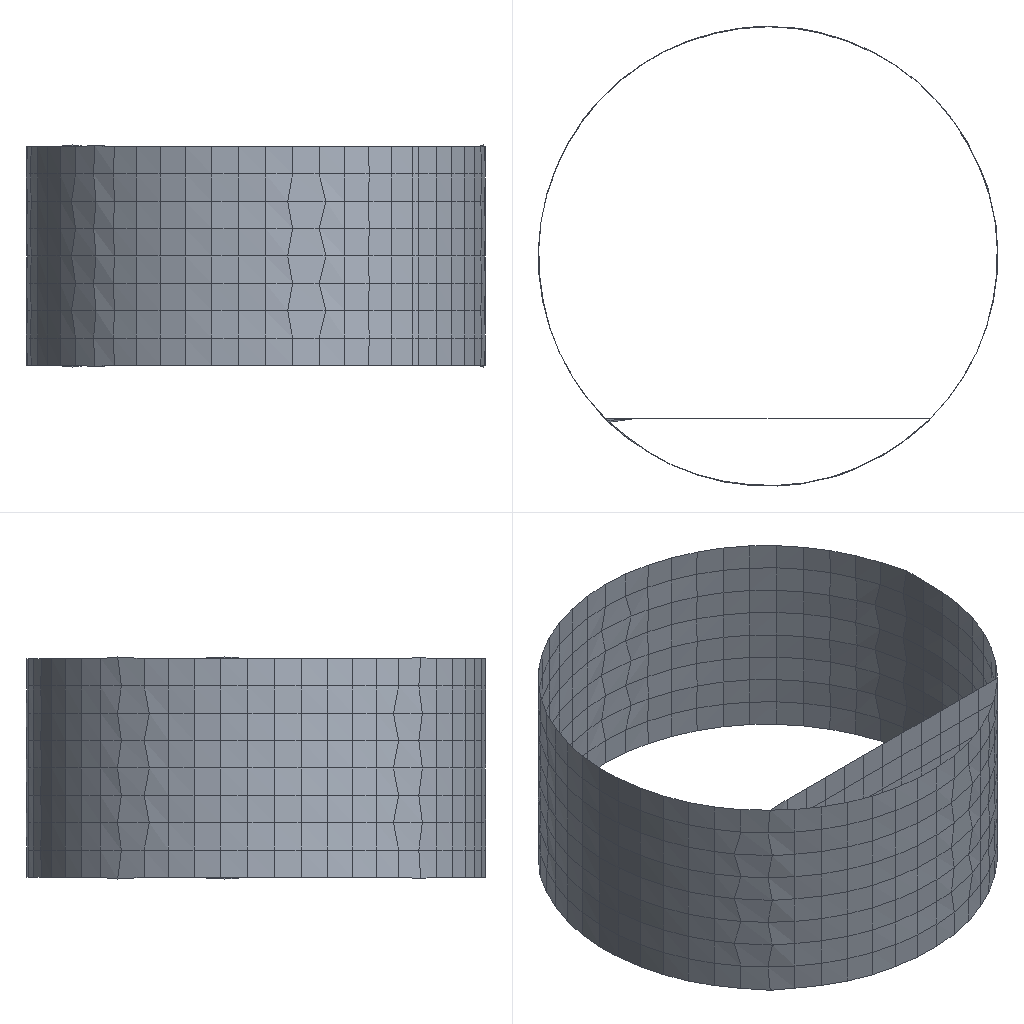Simulation study | abaqus
Set-up summary:
category,name,step,type,value,unit,region
solver,abaqus
solver,version,,,Abaqus/Standard 2020
units,not stated in the deck,,not stated
analysis,deck,,static,static
load_step,Step-1,Step-1,static
load_step,requested,,,1
mesh,nodes,,,1052
mesh,elements,,,966
element_type,B31,,beam,438
element_type,S4R,,shell,528
load,load commands in deck,,count,2
bc,support commands in deck,,count,1
material,FLOOR,,in results
material,FLOOR-STIFFENERS,,in results
material,FRAME,,in results
material,SKIN,,in results
material,STRINGER,,in results
check,setup vs results,,match,"per instance, exact: element labels, types and connectivity; labels of the nodes the elements use; coordinates of those nodes at SINGLE_PRECISION in 17 of 35 instance(s)"
Abaqus input file, long lists of numbers shortened:
*Heading
** Job name: Job-1 Model name: Model-1
** Generated by: Abaqus/CAE 2020
*Preprint, echo=NO, model=NO, history=NO, contact=NO
**
** PARTS
**
*Part, name=Part-1
*Node
      1,  -1484.924,  -1484.924,        2000.
      2,  -1484.924,  -1484.924,           0.
** (583 more lines like these left out)
*Element, type=S4R
  1,   1,   7, 145,  44
  2,   7,   8, 146, 145
** (526 more lines like these left out)
*Nset, nset=Set-1
   1,   2,   3,   4,   5,   6,   7,   8,   9,  10,  11,  12,  13,  14,  15,  16
  17,  18,  19,  20,  21,  22,  23,  24,  25,  26,  27,  28,  29,  30,  31,  32
** (29 more lines like these left out)
*Elset, elset=Set-1, generate
   1,  432,    1
*Nset, nset=Set-2
   1,   2,   4,   6,   7,   8,   9,  10,  11,  12,  13,  26,  27,  28,  29,  30
  31,  32, 123, 124, 125, 126, 127, 128, 129, 130, 131, 132, 133, 134, 135, 136
** (6 more lines like these left out)
*Elset, elset=Set-2, generate
 433,  528,    1
** Section: skin
*Shell Section, elset=Set-1, material=skin
2., 5
** Section: skin
*Shell Section, elset=Set-2, material=skin
2., 5
*End Part
**
*Part, name=floor-stiff
*Node
      1,       -1970.,           0.,           0.
      2,       -1673.,           0.,           0.
** (9 more lines like these left out)
*Element, type=B31
 1,  1,  2
 2,  2,  3
** (8 more lines like these left out)
*Nset, nset=Set-1, generate
  1,  11,   1
*Elset, elset=Set-1, generate
  1,  10,   1
*Nset, nset=Set-3, generate
  1,  11,   1
*Elset, elset=Set-3, generate
  1,  10,   1
** Section: floor-stiff  Profile: Profile-1
*Beam Section, elset=Set-1, material=floor-stiffeners, temperature=GRADIENTS, section=I
0., 50., 40., 30., 4., 4., 4.
0.,0.,-1.
*End Part
**
*Part, name=ring-frame5
*Node
      1,   1763.097,  -1140.828,           0.
      2,    1907.508,  -878.301,           0.
** (42 more lines like these left out)
*Element, type=B31
 1,  1,  2
 2,  2,  3
** (42 more lines like these left out)
*Nset, nset=Set-1, generate
  1,  44,   1
*Elset, elset=Set-1, generate
  1,  44,   1
*Nset, nset=Set-3, generate
  1,  44,   1
*Elset, elset=Set-3, generate
  1,  44,   1
** Section: frame  Profile: frame
*Beam Section, elset=Set-1, material=frame, temperature=GRADIENTS, section=ARBITRARY
3, 50., 158.5, 48.5, 158.5, 3.
1.5, 1.5, 3.
50., 1.5, 3.
0.,0.,-1.
*End Part
**
*Part, name=stringer
*Node
      1,        -600.,           0.,           0.
      2,  -314.286,           0.,           0.
** (6 more lines like these left out)
*Element, type=B31
1, 1, 2
2, 2, 3
** (5 more lines like these left out)
*Nset, nset=Set-1, generate
 1,  8,  1
*Elset, elset=Set-1, generate
 1,  7,  1
*Nset, nset=Set-2, generate
 1,  8,  1
*Elset, elset=Set-2, generate
 1,  7,  1
*Nset, nset=Set-3, generate
 1,  8,  1
*Elset, elset=Set-3, generate
 1,  7,  1
** Section: stringer  Profile: stringer
*Beam Section, elset=Set-1, material=stringer, temperature=GRADIENTS, section=ARBITRARY
3, -22., 35.5, 1., 35.5, 3.
1., -1.5, 2.
24., -1.5, 3.
0.,0.,-1.
*End Part
**
**
** ASSEMBLY
**
*Assembly, name=Assembly
**
*Instance, name=ring-frame5-1, part=ring-frame5
*End Instance
**
*Instance, name=Part-1-1, part=Part-1
*End Instance
**
*Instance, name=ring-frame5-1-lin-2-1, part=ring-frame5
          0.,           0.,         500.
*End Instance
**
*Instance, name=ring-frame5-1-lin-3-1, part=ring-frame5
          0.,           0.,        1000.
*End Instance
**
*Instance, name=ring-frame5-1-lin-4-1, part=ring-frame5
          0.,           0.,        1500.
*End Instance
**
*Instance, name=ring-frame5-1-lin-5-1, part=ring-frame5
          0.,           0.,        2000.
*End Instance
**
*Instance, name=stringer-1, part=stringer
 -1763.097,  1140.828,        1400.
 -1763.097,  1140.828,        1400.,  -1763.097, 1141.828,        1400., 90.
*End Instance
**
*Instance, name=stringer-1-rad-2, part=stringer
-1998.289, 645.632,        1400.
-1998.289, 645.632,        1400., -1998.419, 646.615, 1400.129, 90.976
*End Instance
**
*Instance, name=stringer-1-rad-3, part=stringer
-2097.301, 106.437,        1400.
-2097.301, 106.437,        1400., -2097.551, 107.372, 1400.251, 93.841
*End Instance
**
*Instance, name=stringer-1-rad-4, part=stringer
-2053.385, -440.011,        1400.
-2053.385, -440.011,        1400., -2053.742, -439.148, 1400.357, 98.421
*End Instance
**
*Instance, name=stringer-1-rad-5, part=stringer
-1869.534, -956.473,        1400.
-1869.534, -956.473,        1400., -1869.982, -955.699, 1400.447, 104.478
*End Instance
**
*Instance, name=stringer-1-rad-6, part=stringer
-1558.278, -1407.753,        1400.
-1558.278, -1407.753,        1400., -1558.798, -1407.076, 1400.52, 111.752
*End Instance
**
*Instance, name=stringer-1-rad-7, part=stringer
-1140.828,  -1763.097,        1400.
-1140.828,  -1763.097,        1400., -1141.405, -1762.52, 1400.577,         120.
*End Instance
**
*Instance, name=stringer-1-rad-8, part=stringer
-645.632, -1998.289,        1400.
-645.632, -1998.289,        1400., -646.253, -1997.812, 1400.622, 129.007
*End Instance
**
*Instance, name=stringer-1-rad-9, part=stringer
-106.437, -2097.301,        1400.
-106.437, -2097.301,        1400., -107.092, -2096.923, 1400.655, 138.59
*End Instance
**
*Instance, name=stringer-1-rad-10, part=stringer
440.011, -2053.385,        1400.
440.011, -2053.385,        1400., 439.332, -2053.104, 1400.679, 148.6
*End Instance
**
*Instance, name=stringer-1-rad-11, part=stringer
956.473, -1869.534,        1400.
956.473, -1869.534,        1400., 955.778, -1869.348, 1400.695, 158.909
*End Instance
**
*Instance, name=stringer-1-rad-12, part=stringer
1407.753, -1558.278,        1400.
1407.753, -1558.278,        1400., 1407.049, -1558.185, 1400.704, 169.409
*End Instance
**
*Instance, name=stringer-1-rad-13, part=stringer
  1763.097, -1140.828,        1400.
  1763.097, -1140.828,        1400., 1762.39, -1140.828, 1400.707,         180.
*End Instance
**
*Instance, name=stringer-1-rad-14, part=stringer
1998.289, -645.632,        1400.
1998.289, -645.632,        1400., 1997.585, -645.724, 1400.704, 190.591
*End Instance
**
*Instance, name=stringer-1-rad-15, part=stringer
2097.301, -106.437,        1400.
2097.301, -106.437,        1400., 2096.606, -106.623, 1400.695, 201.091
*End Instance
**
*Instance, name=stringer-1-rad-16, part=stringer
2053.385, 440.011,        1400.
2053.385, 440.011,        1400., 2052.706, 439.73, 1400.679, 211.4
*End Instance
**
*Instance, name=stringer-1-rad-17, part=stringer
1869.534, 956.473,        1400.
1869.534, 956.473,        1400., 1868.88, 956.095, 1400.655, 221.41
*End Instance
**
*Instance, name=stringer-1-rad-18, part=stringer
1558.278, 1407.753,        1400.
1558.278, 1407.753,        1400., 1557.657, 1407.276, 1400.622, 230.993
*End Instance
**
*Instance, name=stringer-1-rad-19, part=stringer
 1140.828,   1763.097,        1400.
 1140.828,   1763.097,        1400., 1140.25, 1762.52, 1400.577,         240.
*End Instance
**
*Instance, name=stringer-1-rad-20, part=stringer
645.632, 1998.289,        1400.
645.632, 1998.289,        1400., 646.152, 1998.967, 1399.48, 111.752
*End Instance
**
*Instance, name=stringer-1-rad-21, part=stringer
106.437, 2097.301,        1400.
106.437, 2097.301,        1400., 106.884, 2098.076, 1399.553, 104.478
*End Instance
**
*Instance, name=stringer-1-rad-22, part=stringer
-440.011, 2053.385,        1400.
-440.011, 2053.385,        1400., -439.654, 2054.248, 1399.643, 98.421
*End Instance
**
*Instance, name=stringer-1-rad-23, part=stringer
-956.473, 1869.534,        1400.
-956.473, 1869.534,        1400., -956.223, 1870.47, 1399.749, 93.841
*End Instance
**
*Instance, name=stringer-1-rad-24, part=stringer
-1407.753, 1558.278,        1400.
-1407.753, 1558.278,        1400., -1407.624, 1559.261, 1399.871, 90.976
*End Instance
**
*Instance, name=floor-stiff-1, part=floor-stiff
   485.076,  -1484.924,        2000.
*End Instance
**
*Instance, name=floor-stiff-1-lin-2-1, part=floor-stiff
   485.076,  -1484.924,        1500.
*End Instance
**
*Instance, name=floor-stiff-1-lin-3-1, part=floor-stiff
   485.076,  -1484.924,        1000.
*End Instance
**
*Instance, name=floor-stiff-1-lin-4-1, part=floor-stiff
   485.076,  -1484.924,         500.
*End Instance
**
*Instance, name=floor-stiff-1-lin-5-1, part=floor-stiff
   485.076,  -1484.924,           0.
*End Instance
**
*Nset, nset=Set-1, instance=floor-stiff-1, generate
  1,  11,   1
*Nset, nset=Set-1, instance=floor-stiff-1-lin-2-1, generate
  1,  11,   1
*Nset, nset=Set-1, instance=floor-stiff-1-lin-4-1, generate
  1,  11,   1
*Nset, nset=Set-1, instance=floor-stiff-1-lin-3-1, generate
  1,  11,   1
*Nset, nset=Set-1, instance=floor-stiff-1-lin-5-1, generate
  1,  11,   1
*Elset, elset=Set-1, instance=floor-stiff-1, generate
  1,  10,   1
*Elset, elset=Set-1, instance=floor-stiff-1-lin-2-1, generate
  1,  10,   1
*Elset, elset=Set-1, instance=floor-stiff-1-lin-4-1, generate
  1,  10,   1
*Elset, elset=Set-1, instance=floor-stiff-1-lin-3-1, generate
  1,  10,   1
*Elset, elset=Set-1, instance=floor-stiff-1-lin-5-1, generate
  1,  10,   1
*Nset, nset=Set-2, instance=Part-1-1
   1,   2,   3,   4,   5,   6,  14,  15,  16,  17,  18,  19,  20,  21,  22,  23
  24,  25,  33,  34,  35,  36,  37,  38,  39,  40,  41,  42,  43,  44,  45,  46
** (7 more lines like these left out)
*Elset, elset=Set-2, instance=Part-1-1
   1,   8,   9,  16,  17,  24,  25,  32,  33,  40,  41,  48,  49,  56,  57,  64
  65,  72,  73,  80,  81,  88,  89,  96,  97, 104, 113, 120, 121, 128, 129, 136
** (7 more lines like these left out)
*Nset, nset=Set-3, instance=Part-1-1, generate
   1,  144,    1
*Elset, elset=Set-3, instance=Part-1-1
   1,   2,   3,   4,   5,   6,   7,   8,   9,  16,  17,  24,  25,  32,  33,  40
  41,  48,  49,  56,  57,  64,  65,  72,  73,  80,  81,  88,  89,  96,  97, 104
** (9 more lines like these left out)
*Elset, elset=_Surf-1_SNEG, internal, instance=Part-1-1, generate
   1,  432,    1
*Surface, type=ELEMENT, name=Surf-1
_Surf-1_SNEG, SNEG
*Elset, elset=_m_Surf-2_, internal, instance=ring-frame5-1, generate
  1,  44,   1
*Elset, elset=_m_Surf-2_, internal, instance=ring-frame5-1-lin-2-1, generate
  1,  44,   1
*Elset, elset=_m_Surf-2_, internal, instance=ring-frame5-1-lin-3-1, generate
  1,  44,   1
*Elset, elset=_m_Surf-2_, internal, instance=stringer-1-rad-2, generate
 1,  7,  1
*Elset, elset=_m_Surf-2_, internal, instance=stringer-1-rad-10, generate
 1,  7,  1
*Elset, elset=_m_Surf-2_, internal, instance=floor-stiff-1-lin-2-1, generate
  1,  10,   1
*Elset, elset=_m_Surf-2_, internal, instance=stringer-1-rad-18, generate
 1,  7,  1
*Elset, elset=_m_Surf-2_, internal, instance=stringer-1-rad-6, generate
 1,  7,  1
*Elset, elset=_m_Surf-2_, internal, instance=stringer-1-rad-14, generate
 1,  7,  1
*Elset, elset=_m_Surf-2_, internal, instance=stringer-1-rad-22, generate
 1,  7,  1
*Elset, elset=_m_Surf-2_, internal, instance=ring-frame5-1-lin-5-1, generate
  1,  44,   1
*Elset, elset=_m_Surf-2_, internal, instance=stringer-1-rad-4, generate
 1,  7,  1
*Elset, elset=_m_Surf-2_, internal, instance=stringer-1-rad-12, generate
 1,  7,  1
*Elset, elset=_m_Surf-2_, internal, instance=floor-stiff-1-lin-4-1, generate
  1,  10,   1
*Elset, elset=_m_Surf-2_, internal, instance=stringer-1-rad-20, generate
 1,  7,  1
*Elset, elset=_m_Surf-2_, internal, instance=stringer-1-rad-8, generate
 1,  7,  1
*Elset, elset=_m_Surf-2_, internal, instance=stringer-1-rad-16, generate
 1,  7,  1
*Elset, elset=_m_Surf-2_, internal, instance=stringer-1-rad-24, generate
 1,  7,  1
*Elset, elset=_m_Surf-2_, internal, instance=ring-frame5-1-lin-4-1, generate
  1,  44,   1
*Elset, elset=_m_Surf-2_, internal, instance=stringer-1-rad-3, generate
 1,  7,  1
*Elset, elset=_m_Surf-2_, internal, instance=stringer-1-rad-11, generate
 1,  7,  1
*Elset, elset=_m_Surf-2_, internal, instance=floor-stiff-1-lin-3-1, generate
  1,  10,   1
*Elset, elset=_m_Surf-2_, internal, instance=stringer-1-rad-19, generate
 1,  7,  1
*Elset, elset=_m_Surf-2_, internal, instance=stringer-1-rad-7, generate
 1,  7,  1
*Elset, elset=_m_Surf-2_, internal, instance=stringer-1-rad-15, generate
 1,  7,  1
*Elset, elset=_m_Surf-2_, internal, instance=stringer-1-rad-23, generate
 1,  7,  1
*Elset, elset=_m_Surf-2_, internal, instance=stringer-1, generate
 1,  7,  1
*Elset, elset=_m_Surf-2_, internal, instance=stringer-1-rad-5, generate
 1,  7,  1
*Elset, elset=_m_Surf-2_, internal, instance=stringer-1-rad-13, generate
 1,  7,  1
*Elset, elset=_m_Surf-2_, internal, instance=floor-stiff-1-lin-5-1, generate
  1,  10,   1
*Elset, elset=_m_Surf-2_, internal, instance=stringer-1-rad-21, generate
 1,  7,  1
*Elset, elset=_m_Surf-2_, internal, instance=stringer-1-rad-9, generate
 1,  7,  1
*Elset, elset=_m_Surf-2_, internal, instance=stringer-1-rad-17, generate
 1,  7,  1
*Elset, elset=_m_Surf-2_, internal, instance=floor-stiff-1, generate
  1,  10,   1
*Surface, type=ELEMENT, name=m_Surf-2
_m_Surf-2_,
*Elset, elset=_s_Surf-2_SNEG, internal, instance=Part-1-1, generate
   1,  528,    1
*Surface, type=ELEMENT, name=s_Surf-2
_s_Surf-2_SNEG, SNEG
** Constraint: Constraint-1
*Tie, name=Constraint-1, adjust=yes
s_Surf-2, m_Surf-2
*End Assembly
*Amplitude, name=Amp-1
             0.,              0.,              1.,              1.
**
** MATERIALS
**
*Material, name=floor
*Elastic
80000., 0.33
*Plastic
450.,0.
*Material, name=floor-stiffeners
*Density
 2.64e-09,
*Elastic
79000., 0.33
*Plastic
455.,0.
*Material, name=frame
*Elastic
77200., 0.33
*Plastic
450.,0.
*Material, name=skin
*Elastic
79000., 0.33
*Plastic
455.,0.
*Material, name=stringer
*Elastic
79000., 0.3
*Plastic
503.,0.
** ----------------------------------------------------------------
**
** STEP: Step-1
**
*Step, name=Step-1, nlgeom=YES, inc=1000
*Static, stabilize=0.0002, allsdtol=0.05, continue=NO
0.01, 1., 1e-05, 1.
**
** BOUNDARY CONDITIONS
**
** Name: BC-1 Type: 对称/反对称/完全固定
*Boundary
Set-3, ENCASTRE
**
** LOADS
**
** Name: Load-1   Type: Pressure
*Dsload, amplitude=Amp-1
Surf-1, P, 0.127
** Name: Load-2   Type: Line load
*Dload, amplitude=Amp-1
Set-1, PY, -5.
**
** OUTPUT REQUESTS
**
*Restart, write, frequency=0
**
** FIELD OUTPUT: F-Output-1
**
*Output, field, variable=PRESELECT
**
** HISTORY OUTPUT: H-Output-1
**
*Output, history, variable=PRESELECT
*End Step
Results summary:
result,step,,completed,increments=12 time=1.0/1.0
result,analysis,,,static
result,last_loadstep,,,1
result,primary field,,,"U, UR"
result,reaction total,,FX,226.073,model units
result,reaction total,,FY,74100.728,model units
result,reaction total,,FZ,-3236.472,model units